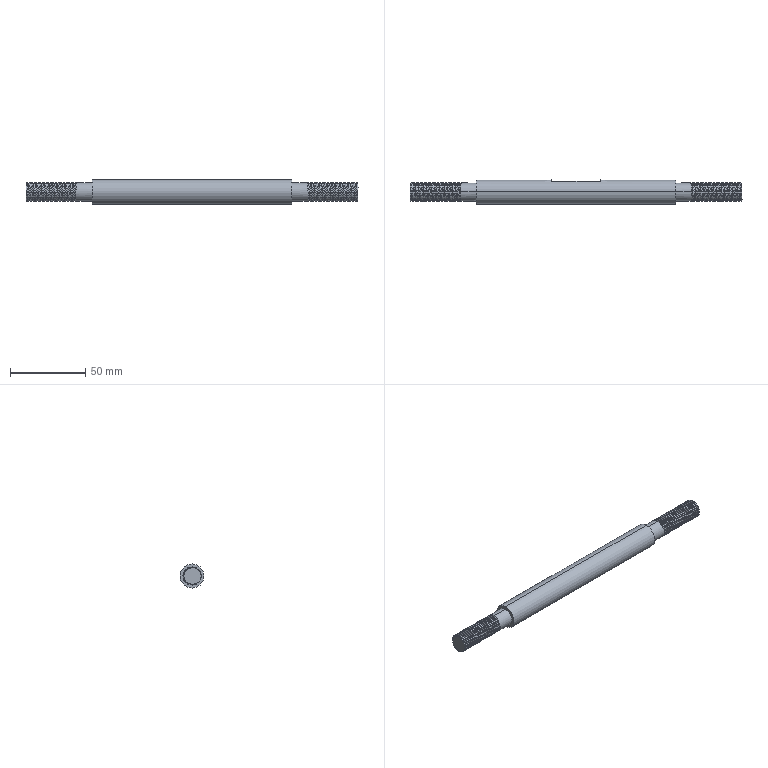Part | SolidWorks | features Helix 1, ICE 1, MirrorPattern 1, Revolution 1, SweepCut 1 | 1 solid | 97 faces | box 221 x 16 x 16 mm | volume 35769 mm3 | cylinder 84 | plane 9 | spline 4 | commonest cylinder face diameters 12 x82 16 x2